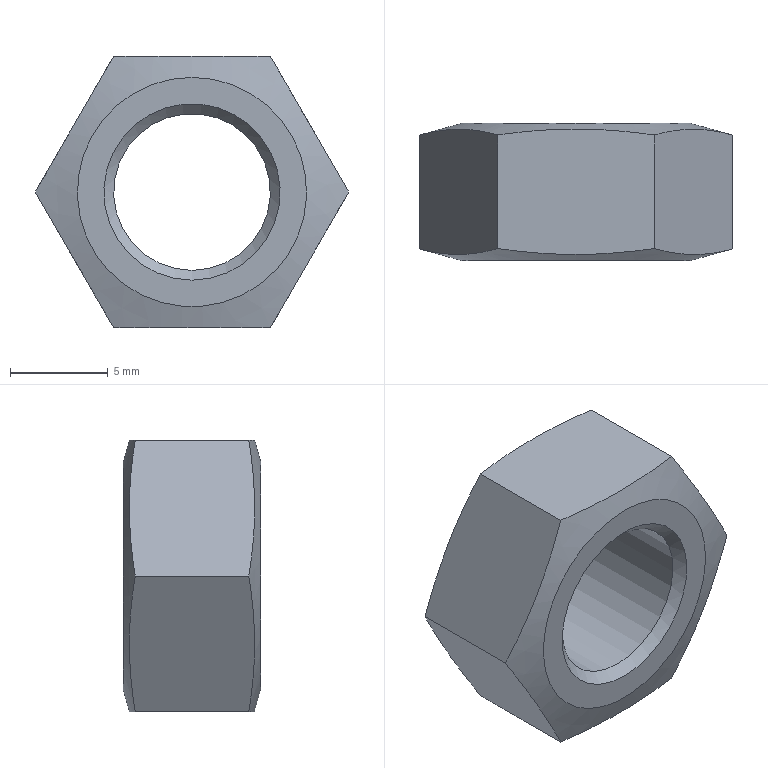Part | STEP file | N108078 | 1 solid | 13 faces | box 16 x 7 x 13.856 mm | volume 779.97 mm3 | plane 8 | cone 4 | cylinder 1 | commonest cylinder face diameters 8 x1